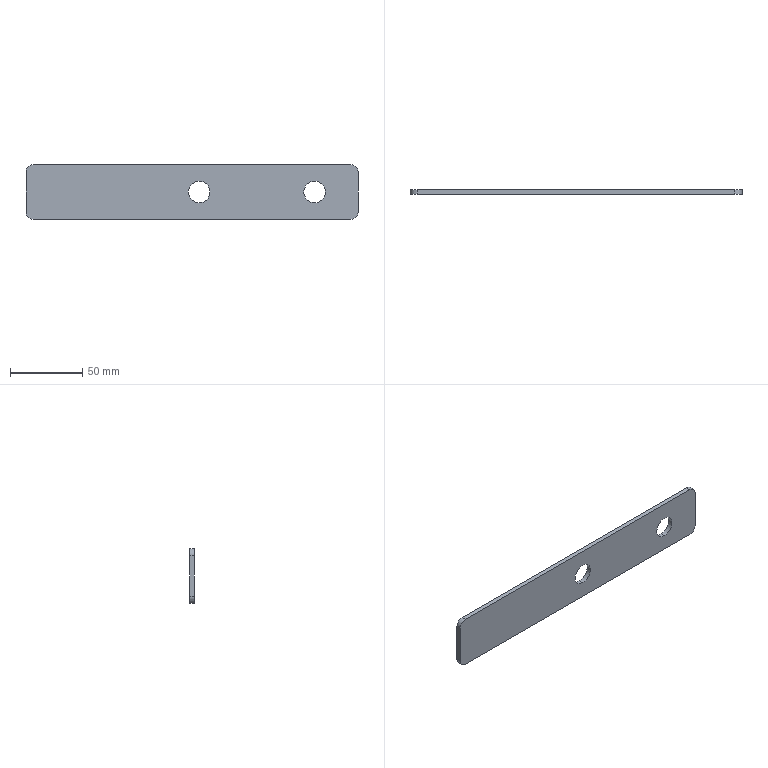Part | SolidWorks | features FlatPattern 1, SMBaseFlange 1, SheetMetal 1 | 1 solid | 14 faces | box 230 x 3.2 x 38 mm | volume 26768 mm3 | cylinder 8 | plane 6 | commonest cylinder face diameters 10 x4 15 x4
STEP:
#1=CARTESIAN_POINT('',(85.,-3.2,-7.5));
#2=VERTEX_POINT('',#1);
#3=CARTESIAN_POINT('',(85.,-3.2,7.5));
#4=VERTEX_POINT('',#3);
#5=CARTESIAN_POINT('',(85.,-3.2,0.));
#6=DIRECTION('',(0.,1.,0.));
#7=DIRECTION('',(0.,0.,1.));
#8=AXIS2_PLACEMENT_3D('',#5,#6,#7);
#9=CIRCLE('',#8,7.5);
#10=EDGE_CURVE('',#2,#4,#9,.T.);
#11=ORIENTED_EDGE('',*,*,#10,.F.);
#12=CARTESIAN_POINT('',(85.,0.,-7.5));
#13=VERTEX_POINT('',#12);
#14=CARTESIAN_POINT('',(85.,-3.2,-7.5));
#15=DIRECTION('',(0.,1.,0.));
#16=VECTOR('',#15,1000.);
#17=LINE('',#14,#16);
#18=EDGE_CURVE('',#2,#13,#17,.T.);
#19=ORIENTED_EDGE('',*,*,#18,.T.);
#20=CARTESIAN_POINT('',(85.,0.,7.5));
#21=VERTEX_POINT('',#20);
#22=CARTESIAN_POINT('',(85.,0.,0.));
#23=DIRECTION('',(0.,1.,0.));
#24=DIRECTION('',(0.,0.,1.));
#25=AXIS2_PLACEMENT_3D('',#22,#23,#24);
#26=CIRCLE('',#25,7.5);
#27=EDGE_CURVE('',#13,#21,#26,.T.);
#28=ORIENTED_EDGE('',*,*,#27,.T.);
#29=CARTESIAN_POINT('',(85.,-3.2,7.5));
#30=DIRECTION('',(0.,1.,0.));
#31=VECTOR('',#30,1000.);
#32=LINE('',#29,#31);
#33=EDGE_CURVE('',#4,#21,#32,.T.);
#34=ORIENTED_EDGE('',*,*,#33,.F.);
#35=EDGE_LOOP('',(#11,#19,#28,#34));
#36=FACE_OUTER_BOUND('',#35,.T.);
#37=CARTESIAN_POINT('',(85.,-3.2,0.));
#38=DIRECTION('',(0.,1.,0.));
#39=DIRECTION('',(0.,0.,1.));
#40=AXIS2_PLACEMENT_3D('',#37,#38,#39);
#41=CYLINDRICAL_SURFACE('',#40,7.5);
#42=ADVANCED_FACE('',(#36),#41,.F.);
#43=CARTESIAN_POINT('',(5.,-3.2,-7.5));
#44=VERTEX_POINT('',#43);
#45=CARTESIAN_POINT('',(5.,-3.2,7.5));
#46=VERTEX_POINT('',#45);
#47=CARTESIAN_POINT('',(5.,-3.2,0.));
#48=DIRECTION('',(0.,1.,0.));
#49=DIRECTION('',(0.,0.,1.));
#50=AXIS2_PLACEMENT_3D('',#47,#48,#49);
#51=CIRCLE('',#50,7.5);
#52=EDGE_CURVE('',#44,#46,#51,.T.);
#53=ORIENTED_EDGE('',*,*,#52,.F.);
#54=CARTESIAN_POINT('',(5.,0.,-7.5));
#55=VERTEX_POINT('',#54);
#56=CARTESIAN_POINT('',(5.,-3.2,-7.5));
#57=DIRECTION('',(0.,1.,0.));
#58=VECTOR('',#57,1000.);
#59=LINE('',#56,#58);
#60=EDGE_CURVE('',#44,#55,#59,.T.);
#61=ORIENTED_EDGE('',*,*,#60,.T.);
#62=CARTESIAN_POINT('',(5.,0.,7.5));
#63=VERTEX_POINT('',#62);
#64=CARTESIAN_POINT('',(5.,0.,0.));
#65=DIRECTION('',(0.,1.,0.));
#66=DIRECTION('',(0.,0.,1.));
#67=AXIS2_PLACEMENT_3D('',#64,#65,#66);
#68=CIRCLE('',#67,7.5);
#69=EDGE_CURVE('',#55,#63,#68,.T.);
#70=ORIENTED_EDGE('',*,*,#69,.T.);
#71=CARTESIAN_POINT('',(5.,-3.2,7.5));
#72=DIRECTION('',(0.,1.,0.));
#73=VECTOR('',#72,1000.);
#74=LINE('',#71,#73);
#75=EDGE_CURVE('',#46,#63,#74,.T.);
#76=ORIENTED_EDGE('',*,*,#75,.F.);
#77=EDGE_LOOP('',(#53,#61,#70,#76));
#78=FACE_OUTER_BOUND('',#77,.T.);
#79=CARTESIAN_POINT('',(5.,-3.2,0.));
#80=DIRECTION('',(0.,1.,0.));
#81=DIRECTION('',(0.,0.,1.));
#82=AXIS2_PLACEMENT_3D('',#79,#80,#81);
#83=CYLINDRICAL_SURFACE('',#82,7.5);
#84=ADVANCED_FACE('',(#78),#83,.F.);
#85=CARTESIAN_POINT('',(110.,0.,19.));
#86=VERTEX_POINT('',#85);
#87=CARTESIAN_POINT('',(115.,0.,14.));
#88=VERTEX_POINT('',#87);
#89=CARTESIAN_POINT('',(110.,0.,14.));
#90=DIRECTION('',(0.,1.,0.));
#91=DIRECTION('',(0.,0.,1.));
#92=AXIS2_PLACEMENT_3D('',#89,#90,#91);
#93=CIRCLE('',#92,5.);
#94=EDGE_CURVE('',#86,#88,#93,.T.);
#95=ORIENTED_EDGE('',*,*,#94,.F.);
#96=CARTESIAN_POINT('',(110.,-3.2,19.));
#97=VERTEX_POINT('',#96);
#98=CARTESIAN_POINT('',(110.,-3.2,19.));
#99=DIRECTION('',(0.,1.,0.));
#100=VECTOR('',#99,1000.);
#101=LINE('',#98,#100);
#102=EDGE_CURVE('',#97,#86,#101,.T.);
#103=ORIENTED_EDGE('',*,*,#102,.F.);
#104=CARTESIAN_POINT('',(115.,-3.2,14.));
#105=VERTEX_POINT('',#104);
#106=CARTESIAN_POINT('',(110.,-3.2,14.));
#107=DIRECTION('',(0.,1.,0.));
#108=DIRECTION('',(0.,0.,1.));
#109=AXIS2_PLACEMENT_3D('',#106,#107,#108);
#110=CIRCLE('',#109,5.);
#111=EDGE_CURVE('',#97,#105,#110,.T.);
#112=ORIENTED_EDGE('',*,*,#111,.T.);
#113=CARTESIAN_POINT('',(115.,-3.2,14.));
#114=DIRECTION('',(0.,1.,0.));
#115=VECTOR('',#114,1000.);
#116=LINE('',#113,#115);
#117=EDGE_CURVE('',#105,#88,#116,.T.);
#118=ORIENTED_EDGE('',*,*,#117,.T.);
#119=EDGE_LOOP('',(#95,#103,#112,#118));
#120=FACE_OUTER_BOUND('',#119,.T.);
#121=CARTESIAN_POINT('',(110.,-3.2,14.));
#122=DIRECTION('',(0.,1.,0.));
#123=DIRECTION('',(0.,0.,1.));
#124=AXIS2_PLACEMENT_3D('',#121,#122,#123);
#125=CYLINDRICAL_SURFACE('',#124,5.);
#126=ADVANCED_FACE('',(#120),#125,.T.);
#127=CARTESIAN_POINT('',(-110.,0.,19.));
#128=VERTEX_POINT('',#127);
#129=CARTESIAN_POINT('',(-110.,0.,19.));
#130=DIRECTION('',(1.,0.,0.));
#131=VECTOR('',#130,1000.);
#132=LINE('',#129,#131);
#133=EDGE_CURVE('',#128,#86,#132,.T.);
#134=ORIENTED_EDGE('',*,*,#133,.F.);
#135=CARTESIAN_POINT('',(-110.,-3.2,19.));
#136=VERTEX_POINT('',#135);
#137=CARTESIAN_POINT('',(-110.,-3.2,19.));
#138=DIRECTION('',(0.,1.,0.));
#139=VECTOR('',#138,1000.);
#140=LINE('',#137,#139);
#141=EDGE_CURVE('',#136,#128,#140,.T.);
#142=ORIENTED_EDGE('',*,*,#141,.F.);
#143=CARTESIAN_POINT('',(-110.,-3.2,19.));
#144=DIRECTION('',(1.,0.,0.));
#145=VECTOR('',#144,1000.);
#146=LINE('',#143,#145);
#147=EDGE_CURVE('',#136,#97,#146,.T.);
#148=ORIENTED_EDGE('',*,*,#147,.T.);
#149=ORIENTED_EDGE('',*,*,#102,.T.);
#150=EDGE_LOOP('',(#134,#142,#148,#149));
#151=FACE_OUTER_BOUND('',#150,.T.);
#152=CARTESIAN_POINT('',(-110.,-3.2,19.));
#153=DIRECTION('',(0.,0.,1.));
#154=DIRECTION('',(1.,0.,0.));
#155=AXIS2_PLACEMENT_3D('',#152,#153,#154);
#156=PLANE('',#155);
#157=ADVANCED_FACE('',(#151),#156,.T.);
#158=CARTESIAN_POINT('',(-115.,0.,14.));
#159=VERTEX_POINT('',#158);
#160=CARTESIAN_POINT('',(-110.,0.,14.));
#161=DIRECTION('',(0.,1.,0.));
#162=DIRECTION('',(0.,0.,1.));
#163=AXIS2_PLACEMENT_3D('',#160,#161,#162);
#164=CIRCLE('',#163,5.);
#165=EDGE_CURVE('',#159,#128,#164,.T.);
#166=ORIENTED_EDGE('',*,*,#165,.F.);
#167=CARTESIAN_POINT('',(-115.,-3.2,14.));
#168=VERTEX_POINT('',#167);
#169=CARTESIAN_POINT('',(-115.,-3.2,14.));
#170=DIRECTION('',(0.,1.,0.));
#171=VECTOR('',#170,1000.);
#172=LINE('',#169,#171);
#173=EDGE_CURVE('',#168,#159,#172,.T.);
#174=ORIENTED_EDGE('',*,*,#173,.F.);
#175=CARTESIAN_POINT('',(-110.,-3.2,14.));
#176=DIRECTION('',(0.,1.,0.));
#177=DIRECTION('',(0.,0.,1.));
#178=AXIS2_PLACEMENT_3D('',#175,#176,#177);
#179=CIRCLE('',#178,5.);
#180=EDGE_CURVE('',#168,#136,#179,.T.);
#181=ORIENTED_EDGE('',*,*,#180,.T.);
#182=ORIENTED_EDGE('',*,*,#141,.T.);
#183=EDGE_LOOP('',(#166,#174,#181,#182));
#184=FACE_OUTER_BOUND('',#183,.T.);
#185=CARTESIAN_POINT('',(-110.,-3.2,14.));
#186=DIRECTION('',(0.,1.,0.));
#187=DIRECTION('',(0.,0.,1.));
#188=AXIS2_PLACEMENT_3D('',#185,#186,#187);
#189=CYLINDRICAL_SURFACE('',#188,5.);
#190=ADVANCED_FACE('',(#184),#189,.T.);
#191=CARTESIAN_POINT('',(-115.,0.,-14.));
#192=VERTEX_POINT('',#191);
#193=CARTESIAN_POINT('',(-115.,0.,-14.));
#194=DIRECTION('',(0.,0.,1.));
#195=VECTOR('',#194,1000.);
#196=LINE('',#193,#195);
#197=EDGE_CURVE('',#192,#159,#196,.T.);
#198=ORIENTED_EDGE('',*,*,#197,.F.);
#199=CARTESIAN_POINT('',(-115.,-3.2,-14.));
#200=VERTEX_POINT('',#199);
#201=CARTESIAN_POINT('',(-115.,-3.2,-14.));
#202=DIRECTION('',(0.,1.,0.));
#203=VECTOR('',#202,1000.);
#204=LINE('',#201,#203);
#205=EDGE_CURVE('',#200,#192,#204,.T.);
#206=ORIENTED_EDGE('',*,*,#205,.F.);
#207=CARTESIAN_POINT('',(-115.,-3.2,-14.));
#208=DIRECTION('',(0.,0.,1.));
#209=VECTOR('',#208,1000.);
#210=LINE('',#207,#209);
#211=EDGE_CURVE('',#200,#168,#210,.T.);
#212=ORIENTED_EDGE('',*,*,#211,.T.);
#213=ORIENTED_EDGE('',*,*,#173,.T.);
#214=EDGE_LOOP('',(#198,#206,#212,#213));
#215=FACE_OUTER_BOUND('',#214,.T.);
#216=CARTESIAN_POINT('',(-115.,-3.2,-14.));
#217=DIRECTION('',(-1.,0.,0.));
#218=DIRECTION('',(0.,0.,1.));
#219=AXIS2_PLACEMENT_3D('',#216,#217,#218);
#220=PLANE('',#219);
#221=ADVANCED_FACE('',(#215),#220,.T.);
#222=CARTESIAN_POINT('',(-110.,0.,-19.));
#223=VERTEX_POINT('',#222);
#224=CARTESIAN_POINT('',(-110.,0.,-14.));
#225=DIRECTION('',(0.,1.,0.));
#226=DIRECTION('',(0.,0.,1.));
#227=AXIS2_PLACEMENT_3D('',#224,#225,#226);
#228=CIRCLE('',#227,5.);
#229=EDGE_CURVE('',#223,#192,#228,.T.);
#230=ORIENTED_EDGE('',*,*,#229,.F.);
#231=CARTESIAN_POINT('',(-110.,-3.2,-19.));
#232=VERTEX_POINT('',#231);
#233=CARTESIAN_POINT('',(-110.,-3.2,-19.));
#234=DIRECTION('',(0.,1.,0.));
#235=VECTOR('',#234,1000.);
#236=LINE('',#233,#235);
#237=EDGE_CURVE('',#232,#223,#236,.T.);
#238=ORIENTED_EDGE('',*,*,#237,.F.);
#239=CARTESIAN_POINT('',(-110.,-3.2,-14.));
#240=DIRECTION('',(0.,1.,0.));
#241=DIRECTION('',(0.,0.,1.));
#242=AXIS2_PLACEMENT_3D('',#239,#240,#241);
#243=CIRCLE('',#242,5.);
#244=EDGE_CURVE('',#232,#200,#243,.T.);
#245=ORIENTED_EDGE('',*,*,#244,.T.);
#246=ORIENTED_EDGE('',*,*,#205,.T.);
#247=EDGE_LOOP('',(#230,#238,#245,#246));
#248=FACE_OUTER_BOUND('',#247,.T.);
#249=CARTESIAN_POINT('',(-110.,-3.2,-14.));
#250=DIRECTION('',(0.,1.,0.));
#251=DIRECTION('',(0.,0.,1.));
#252=AXIS2_PLACEMENT_3D('',#249,#250,#251);
#253=CYLINDRICAL_SURFACE('',#252,5.);
#254=ADVANCED_FACE('',(#248),#253,.T.);
#255=CARTESIAN_POINT('',(110.,0.,-19.));
#256=VERTEX_POINT('',#255);
#257=CARTESIAN_POINT('',(-110.,0.,-19.));
#258=DIRECTION('',(-1.,0.,0.));
#259=VECTOR('',#258,1000.);
#260=LINE('',#257,#259);
#261=EDGE_CURVE('',#256,#223,#260,.T.);
#262=ORIENTED_EDGE('',*,*,#261,.F.);
#263=CARTESIAN_POINT('',(110.,-3.2,-19.));
#264=VERTEX_POINT('',#263);
#265=CARTESIAN_POINT('',(110.,-3.2,-19.));
#266=DIRECTION('',(0.,1.,0.));
#267=VECTOR('',#266,1000.);
#268=LINE('',#265,#267);
#269=EDGE_CURVE('',#264,#256,#268,.T.);
#270=ORIENTED_EDGE('',*,*,#269,.F.);
#271=CARTESIAN_POINT('',(-110.,-3.2,-19.));
#272=DIRECTION('',(-1.,0.,0.));
#273=VECTOR('',#272,1000.);
#274=LINE('',#271,#273);
#275=EDGE_CURVE('',#264,#232,#274,.T.);
#276=ORIENTED_EDGE('',*,*,#275,.T.);
#277=ORIENTED_EDGE('',*,*,#237,.T.);
#278=EDGE_LOOP('',(#262,#270,#276,#277));
#279=FACE_OUTER_BOUND('',#278,.T.);
#280=CARTESIAN_POINT('',(-110.,-3.2,-19.));
#281=DIRECTION('',(0.,0.,-1.));
#282=DIRECTION('',(-1.,0.,0.));
#283=AXIS2_PLACEMENT_3D('',#280,#281,#282);
#284=PLANE('',#283);
#285=ADVANCED_FACE('',(#279),#284,.T.);
#286=CARTESIAN_POINT('',(115.,0.,-14.));
#287=VERTEX_POINT('',#286);
#288=CARTESIAN_POINT('',(110.,0.,-14.));
#289=DIRECTION('',(0.,1.,0.));
#290=DIRECTION('',(0.,0.,-1.));
#291=AXIS2_PLACEMENT_3D('',#288,#289,#290);
#292=CIRCLE('',#291,5.);
#293=EDGE_CURVE('',#287,#256,#292,.T.);
#294=ORIENTED_EDGE('',*,*,#293,.F.);
#295=CARTESIAN_POINT('',(115.,-3.2,-14.));
#296=VERTEX_POINT('',#295);
#297=CARTESIAN_POINT('',(115.,-3.2,-14.));
#298=DIRECTION('',(0.,1.,0.));
#299=VECTOR('',#298,1000.);
#300=LINE('',#297,#299);
#301=EDGE_CURVE('',#296,#287,#300,.T.);
#302=ORIENTED_EDGE('',*,*,#301,.F.);
#303=CARTESIAN_POINT('',(110.,-3.2,-14.));
#304=DIRECTION('',(0.,1.,0.));
#305=DIRECTION('',(0.,0.,-1.));
#306=AXIS2_PLACEMENT_3D('',#303,#304,#305);
#307=CIRCLE('',#306,5.);
#308=EDGE_CURVE('',#296,#264,#307,.T.);
#309=ORIENTED_EDGE('',*,*,#308,.T.);
#310=ORIENTED_EDGE('',*,*,#269,.T.);
#311=EDGE_LOOP('',(#294,#302,#309,#310));
#312=FACE_OUTER_BOUND('',#311,.T.);
#313=CARTESIAN_POINT('',(110.,-3.2,-14.));
#314=DIRECTION('',(0.,1.,0.));
#315=DIRECTION('',(0.,0.,1.));
#316=AXIS2_PLACEMENT_3D('',#313,#314,#315);
#317=CYLINDRICAL_SURFACE('',#316,5.);
#318=ADVANCED_FACE('',(#312),#317,.T.);
#319=CARTESIAN_POINT('',(115.,0.,-14.));
#320=DIRECTION('',(0.,0.,-1.));
#321=VECTOR('',#320,1000.);
#322=LINE('',#319,#321);
#323=EDGE_CURVE('',#88,#287,#322,.T.);
#324=ORIENTED_EDGE('',*,*,#323,.F.);
#325=ORIENTED_EDGE('',*,*,#117,.F.);
#326=CARTESIAN_POINT('',(115.,-3.2,-14.));
#327=DIRECTION('',(0.,0.,-1.));
#328=VECTOR('',#327,1000.);
#329=LINE('',#326,#328);
#330=EDGE_CURVE('',#105,#296,#329,.T.);
#331=ORIENTED_EDGE('',*,*,#330,.T.);
#332=ORIENTED_EDGE('',*,*,#301,.T.);
#333=EDGE_LOOP('',(#324,#325,#331,#332));
#334=FACE_OUTER_BOUND('',#333,.T.);
#335=CARTESIAN_POINT('',(115.,-3.2,-14.));
#336=DIRECTION('',(1.,0.,0.));
#337=DIRECTION('',(0.,0.,-1.));
#338=AXIS2_PLACEMENT_3D('',#335,#336,#337);
#339=PLANE('',#338);
#340=ADVANCED_FACE('',(#334),#339,.T.);
#341=CARTESIAN_POINT('',(85.,-3.2,0.));
#342=DIRECTION('',(0.,1.,0.));
#343=DIRECTION('',(0.,0.,1.));
#344=AXIS2_PLACEMENT_3D('',#341,#342,#343);
#345=CIRCLE('',#344,7.5);
#346=EDGE_CURVE('',#4,#2,#345,.T.);
#347=ORIENTED_EDGE('',*,*,#346,.T.);
#348=ORIENTED_EDGE('',*,*,#10,.T.);
#349=EDGE_LOOP('',(#347,#348));
#350=FACE_BOUND('',#349,.T.);
#351=CARTESIAN_POINT('',(5.,-3.2,0.));
#352=DIRECTION('',(0.,1.,0.));
#353=DIRECTION('',(0.,0.,1.));
#354=AXIS2_PLACEMENT_3D('',#351,#352,#353);
#355=CIRCLE('',#354,7.5);
#356=EDGE_CURVE('',#46,#44,#355,.T.);
#357=ORIENTED_EDGE('',*,*,#356,.T.);
#358=ORIENTED_EDGE('',*,*,#52,.T.);
#359=EDGE_LOOP('',(#357,#358));
#360=FACE_BOUND('',#359,.T.);
#361=ORIENTED_EDGE('',*,*,#111,.F.);
#362=ORIENTED_EDGE('',*,*,#147,.F.);
#363=ORIENTED_EDGE('',*,*,#180,.F.);
#364=ORIENTED_EDGE('',*,*,#211,.F.);
#365=ORIENTED_EDGE('',*,*,#244,.F.);
#366=ORIENTED_EDGE('',*,*,#275,.F.);
#367=ORIENTED_EDGE('',*,*,#308,.F.);
#368=ORIENTED_EDGE('',*,*,#330,.F.);
#369=EDGE_LOOP('',(#361,#362,#363,#364,#365,#366,#367,#368));
#370=FACE_OUTER_BOUND('',#369,.T.);
#371=CARTESIAN_POINT('',(110.,-3.2,14.));
#372=DIRECTION('',(0.,1.,0.));
#373=DIRECTION('',(0.,0.,1.));
#374=AXIS2_PLACEMENT_3D('',#371,#372,#373);
#375=PLANE('',#374);
#376=ADVANCED_FACE('',(#350,#360,#370),#375,.F.);
#377=CARTESIAN_POINT('',(85.,0.,0.));
#378=DIRECTION('',(0.,1.,0.));
#379=DIRECTION('',(0.,0.,1.));
#380=AXIS2_PLACEMENT_3D('',#377,#378,#379);
#381=CIRCLE('',#380,7.5);
#382=EDGE_CURVE('',#21,#13,#381,.T.);
#383=ORIENTED_EDGE('',*,*,#382,.F.);
#384=ORIENTED_EDGE('',*,*,#27,.F.);
#385=EDGE_LOOP('',(#383,#384));
#386=FACE_BOUND('',#385,.T.);
#387=CARTESIAN_POINT('',(5.,0.,0.));
#388=DIRECTION('',(0.,1.,0.));
#389=DIRECTION('',(0.,0.,1.));
#390=AXIS2_PLACEMENT_3D('',#387,#388,#389);
#391=CIRCLE('',#390,7.5);
#392=EDGE_CURVE('',#63,#55,#391,.T.);
#393=ORIENTED_EDGE('',*,*,#392,.F.);
#394=ORIENTED_EDGE('',*,*,#69,.F.);
#395=EDGE_LOOP('',(#393,#394));
#396=FACE_BOUND('',#395,.T.);
#397=ORIENTED_EDGE('',*,*,#94,.T.);
#398=ORIENTED_EDGE('',*,*,#323,.T.);
#399=ORIENTED_EDGE('',*,*,#293,.T.);
#400=ORIENTED_EDGE('',*,*,#261,.T.);
#401=ORIENTED_EDGE('',*,*,#229,.T.);
#402=ORIENTED_EDGE('',*,*,#197,.T.);
#403=ORIENTED_EDGE('',*,*,#165,.T.);
#404=ORIENTED_EDGE('',*,*,#133,.T.);
#405=EDGE_LOOP('',(#397,#398,#399,#400,#401,#402,#403,#404));
#406=FACE_OUTER_BOUND('',#405,.T.);
#407=CARTESIAN_POINT('',(110.,0.,14.));
#408=DIRECTION('',(0.,1.,0.));
#409=DIRECTION('',(0.,0.,1.));
#410=AXIS2_PLACEMENT_3D('',#407,#408,#409);
#411=PLANE('',#410);
#412=ADVANCED_FACE('',(#386,#396,#406),#411,.T.);
#413=ORIENTED_EDGE('',*,*,#60,.F.);
#414=ORIENTED_EDGE('',*,*,#356,.F.);
#415=ORIENTED_EDGE('',*,*,#75,.T.);
#416=ORIENTED_EDGE('',*,*,#392,.T.);
#417=EDGE_LOOP('',(#413,#414,#415,#416));
#418=FACE_OUTER_BOUND('',#417,.T.);
#419=CARTESIAN_POINT('',(5.,-3.2,0.));
#420=DIRECTION('',(0.,1.,0.));
#421=DIRECTION('',(0.,0.,1.));
#422=AXIS2_PLACEMENT_3D('',#419,#420,#421);
#423=CYLINDRICAL_SURFACE('',#422,7.5);
#424=ADVANCED_FACE('',(#418),#423,.F.);
#425=ORIENTED_EDGE('',*,*,#18,.F.);
#426=ORIENTED_EDGE('',*,*,#346,.F.);
#427=ORIENTED_EDGE('',*,*,#33,.T.);
#428=ORIENTED_EDGE('',*,*,#382,.T.);
#429=EDGE_LOOP('',(#425,#426,#427,#428));
#430=FACE_OUTER_BOUND('',#429,.T.);
#431=CARTESIAN_POINT('',(85.,-3.2,0.));
#432=DIRECTION('',(0.,1.,0.));
#433=DIRECTION('',(0.,0.,1.));
#434=AXIS2_PLACEMENT_3D('',#431,#432,#433);
#435=CYLINDRICAL_SURFACE('',#434,7.5);
#436=ADVANCED_FACE('',(#430),#435,.F.);
#437=CLOSED_SHELL('',(#42,#84,#126,#157,#190,#221,#254,#285,#318,#340,#376,#412,#424,#436));
#438=MANIFOLD_SOLID_BREP('',#437);
#439=CARTESIAN_POINT('',(0.,0.,0.));
#440=DIRECTION('',(0.,0.,1.));
#441=DIRECTION('',(1.,0.,0.));
#442=AXIS2_PLACEMENT_3D('',#439,#440,#441);
#443=(LENGTH_UNIT()NAMED_UNIT(*)SI_UNIT(.MILLI.,.METRE.));
#444=UNCERTAINTY_MEASURE_WITH_UNIT(LENGTH_MEASURE(0.00001),#443,'','');
#445=(NAMED_UNIT(*)PLANE_ANGLE_UNIT()SI_UNIT($,.RADIAN.));
#446=(NAMED_UNIT(*)SI_UNIT($,.STERADIAN.)SOLID_ANGLE_UNIT());
#447=(GEOMETRIC_REPRESENTATION_CONTEXT(3)GLOBAL_UNCERTAINTY_ASSIGNED_CONTEXT((#444))GLOBAL_UNIT_ASSIGNED_CONTEXT((#443,#445,#446))REPRESENTATION_CONTEXT('',''));
#448=ADVANCED_BREP_SHAPE_REPRESENTATION('',(#438,#442),#447);